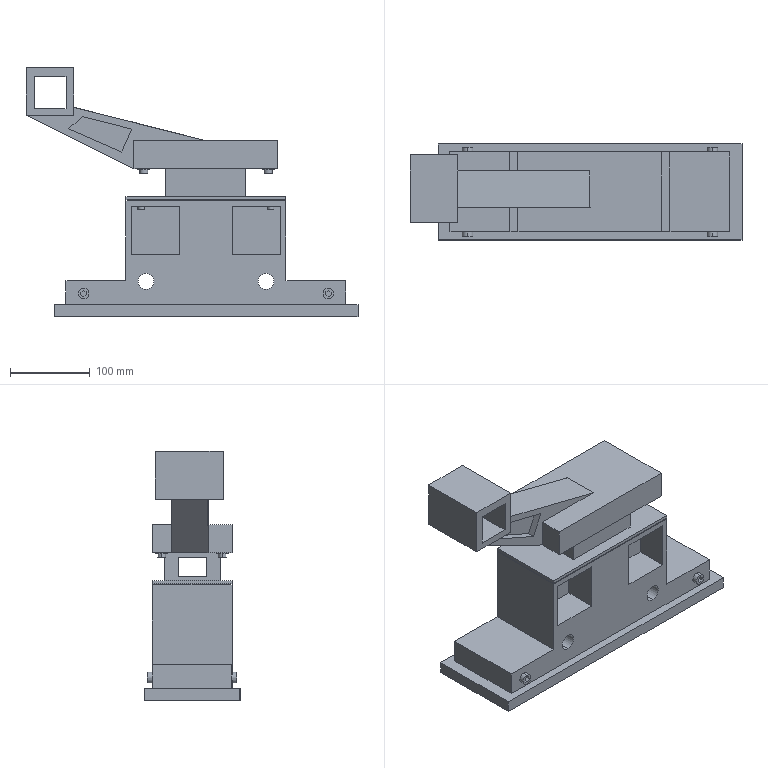Part | SolidWorks | features ICE 14, MirrorPattern 9, Extrusion 1 | 1 solid | 221 faces | box 415 x 120 x 311.384 mm | volume 4368887 mm3 | plane 185 | cylinder 36 | commonest cylinder face diameters 8 x8 10.1 x8 13.426 x8 15 x8 20 x4